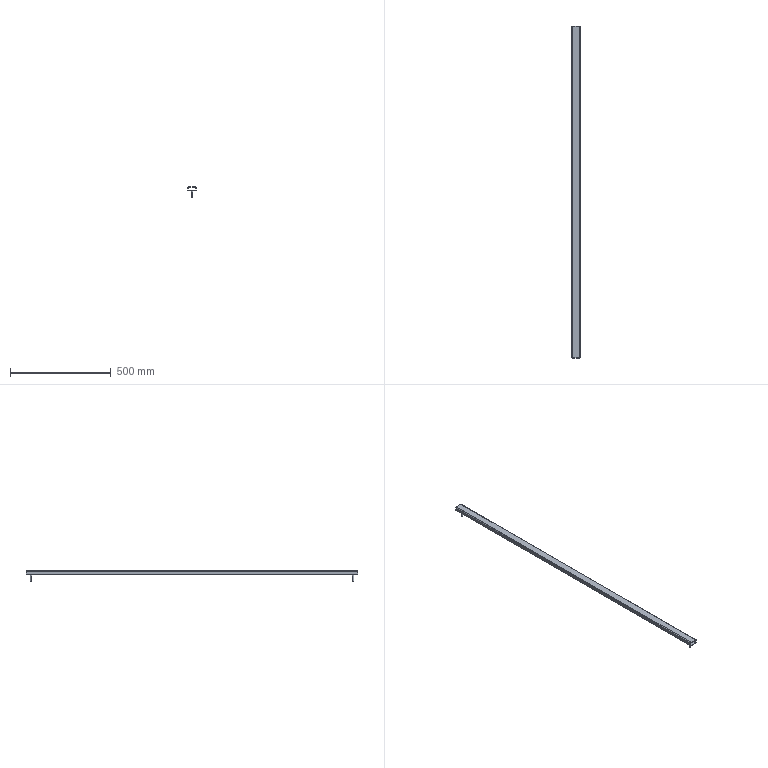Part | SolidWorks | features Extrusion 1, ICE 1 | 1 solid | 24 faces | box 40 x 1650 x 50 mm | volume 355619 mm3 | cylinder 12 | plane 12 | commonest cylinder face diameters 8 x8 4 x4
STEP:
#1=CARTESIAN_POINT('',(-4.,25.,-40.));
#2=VERTEX_POINT('',#1);
#3=CARTESIAN_POINT('',(4.,25.,-40.));
#4=VERTEX_POINT('',#3);
#5=CARTESIAN_POINT('',(0.,25.,-40.));
#6=DIRECTION('',(0.,0.,-1.));
#7=DIRECTION('',(-1.,0.,0.));
#8=AXIS2_PLACEMENT_3D('',#5,#6,#7);
#9=CIRCLE('',#8,4.);
#10=EDGE_CURVE('',#2,#4,#9,.T.);
#11=ORIENTED_EDGE('',*,*,#10,.F.);
#12=CARTESIAN_POINT('',(-4.,25.,-10.));
#13=VERTEX_POINT('',#12);
#14=CARTESIAN_POINT('',(-4.,25.,-40.));
#15=DIRECTION('',(0.,0.,1.));
#16=VECTOR('',#15,1000.);
#17=LINE('',#14,#16);
#18=EDGE_CURVE('',#2,#13,#17,.T.);
#19=ORIENTED_EDGE('',*,*,#18,.T.);
#20=CARTESIAN_POINT('',(4.,25.,-10.));
#21=VERTEX_POINT('',#20);
#22=CARTESIAN_POINT('',(0.,25.,-10.));
#23=DIRECTION('',(0.,0.,-1.));
#24=DIRECTION('',(1.,0.,0.));
#25=AXIS2_PLACEMENT_3D('',#22,#23,#24);
#26=CIRCLE('',#25,4.);
#27=EDGE_CURVE('',#13,#21,#26,.T.);
#28=ORIENTED_EDGE('',*,*,#27,.T.);
#29=CARTESIAN_POINT('',(4.,25.,-40.));
#30=DIRECTION('',(0.,0.,1.));
#31=VECTOR('',#30,1000.);
#32=LINE('',#29,#31);
#33=EDGE_CURVE('',#4,#21,#32,.T.);
#34=ORIENTED_EDGE('',*,*,#33,.F.);
#35=EDGE_LOOP('',(#11,#19,#28,#34));
#36=FACE_OUTER_BOUND('',#35,.T.);
#37=CARTESIAN_POINT('',(0.,25.,-40.));
#38=DIRECTION('',(0.,0.,1.));
#39=DIRECTION('',(1.,0.,0.));
#40=AXIS2_PLACEMENT_3D('',#37,#38,#39);
#41=CYLINDRICAL_SURFACE('',#40,4.);
#42=ADVANCED_FACE('',(#36),#41,.T.);
#43=CARTESIAN_POINT('',(-4.,1625.,-40.));
#44=VERTEX_POINT('',#43);
#45=CARTESIAN_POINT('',(4.,1625.,-40.));
#46=VERTEX_POINT('',#45);
#47=CARTESIAN_POINT('',(0.,1625.,-40.));
#48=DIRECTION('',(0.,0.,-1.));
#49=DIRECTION('',(-1.,0.,0.));
#50=AXIS2_PLACEMENT_3D('',#47,#48,#49);
#51=CIRCLE('',#50,4.);
#52=EDGE_CURVE('',#44,#46,#51,.T.);
#53=ORIENTED_EDGE('',*,*,#52,.F.);
#54=CARTESIAN_POINT('',(-4.,1625.,-10.));
#55=VERTEX_POINT('',#54);
#56=CARTESIAN_POINT('',(-4.,1625.,-40.));
#57=DIRECTION('',(0.,0.,1.));
#58=VECTOR('',#57,1000.);
#59=LINE('',#56,#58);
#60=EDGE_CURVE('',#44,#55,#59,.T.);
#61=ORIENTED_EDGE('',*,*,#60,.T.);
#62=CARTESIAN_POINT('',(4.,1625.,-10.));
#63=VERTEX_POINT('',#62);
#64=CARTESIAN_POINT('',(0.,1625.,-10.));
#65=DIRECTION('',(0.,0.,-1.));
#66=DIRECTION('',(1.,0.,0.));
#67=AXIS2_PLACEMENT_3D('',#64,#65,#66);
#68=CIRCLE('',#67,4.);
#69=EDGE_CURVE('',#55,#63,#68,.T.);
#70=ORIENTED_EDGE('',*,*,#69,.T.);
#71=CARTESIAN_POINT('',(4.,1625.,-40.));
#72=DIRECTION('',(0.,0.,1.));
#73=VECTOR('',#72,1000.);
#74=LINE('',#71,#73);
#75=EDGE_CURVE('',#46,#63,#74,.T.);
#76=ORIENTED_EDGE('',*,*,#75,.F.);
#77=EDGE_LOOP('',(#53,#61,#70,#76));
#78=FACE_OUTER_BOUND('',#77,.T.);
#79=CARTESIAN_POINT('',(0.,1625.,-40.));
#80=DIRECTION('',(0.,0.,1.));
#81=DIRECTION('',(1.,0.,0.));
#82=AXIS2_PLACEMENT_3D('',#79,#80,#81);
#83=CYLINDRICAL_SURFACE('',#82,4.);
#84=ADVANCED_FACE('',(#78),#83,.T.);
#85=CARTESIAN_POINT('',(-20.,1650.,6.));
#86=VERTEX_POINT('',#85);
#87=CARTESIAN_POINT('',(-16.,1650.,10.));
#88=VERTEX_POINT('',#87);
#89=CARTESIAN_POINT('',(-16.,1650.,6.));
#90=DIRECTION('',(0.,1.,0.));
#91=DIRECTION('',(0.,0.,-1.));
#92=AXIS2_PLACEMENT_3D('',#89,#90,#91);
#93=CIRCLE('',#92,4.);
#94=EDGE_CURVE('',#86,#88,#93,.T.);
#95=ORIENTED_EDGE('',*,*,#94,.T.);
#96=CARTESIAN_POINT('',(16.,1650.,10.));
#97=VERTEX_POINT('',#96);
#98=CARTESIAN_POINT('',(-16.,1650.,10.));
#99=DIRECTION('',(1.,0.,0.));
#100=VECTOR('',#99,1000.);
#101=LINE('',#98,#100);
#102=EDGE_CURVE('',#88,#97,#101,.T.);
#103=ORIENTED_EDGE('',*,*,#102,.T.);
#104=CARTESIAN_POINT('',(20.,1650.,6.));
#105=VERTEX_POINT('',#104);
#106=CARTESIAN_POINT('',(16.,1650.,6.));
#107=DIRECTION('',(0.,1.,0.));
#108=DIRECTION('',(0.,0.,1.));
#109=AXIS2_PLACEMENT_3D('',#106,#107,#108);
#110=CIRCLE('',#109,4.);
#111=EDGE_CURVE('',#97,#105,#110,.T.);
#112=ORIENTED_EDGE('',*,*,#111,.T.);
#113=CARTESIAN_POINT('',(20.,1650.,-6.));
#114=VERTEX_POINT('',#113);
#115=CARTESIAN_POINT('',(20.,1650.,6.));
#116=DIRECTION('',(0.,0.,-1.));
#117=VECTOR('',#116,1000.);
#118=LINE('',#115,#117);
#119=EDGE_CURVE('',#105,#114,#118,.T.);
#120=ORIENTED_EDGE('',*,*,#119,.T.);
#121=CARTESIAN_POINT('',(16.,1650.,-10.));
#122=VERTEX_POINT('',#121);
#123=CARTESIAN_POINT('',(16.,1650.,-6.));
#124=DIRECTION('',(0.,1.,0.));
#125=DIRECTION('',(0.,0.,-1.));
#126=AXIS2_PLACEMENT_3D('',#123,#124,#125);
#127=CIRCLE('',#126,4.);
#128=EDGE_CURVE('',#114,#122,#127,.T.);
#129=ORIENTED_EDGE('',*,*,#128,.T.);
#130=CARTESIAN_POINT('',(-16.,1650.,-10.));
#131=VERTEX_POINT('',#130);
#132=CARTESIAN_POINT('',(-16.,1650.,-10.));
#133=DIRECTION('',(-1.,0.,0.));
#134=VECTOR('',#133,1000.);
#135=LINE('',#132,#134);
#136=EDGE_CURVE('',#122,#131,#135,.T.);
#137=ORIENTED_EDGE('',*,*,#136,.T.);
#138=CARTESIAN_POINT('',(-20.,1650.,-6.));
#139=VERTEX_POINT('',#138);
#140=CARTESIAN_POINT('',(-16.,1650.,-6.));
#141=DIRECTION('',(0.,1.,0.));
#142=DIRECTION('',(0.,0.,-1.));
#143=AXIS2_PLACEMENT_3D('',#140,#141,#142);
#144=CIRCLE('',#143,4.);
#145=EDGE_CURVE('',#131,#139,#144,.T.);
#146=ORIENTED_EDGE('',*,*,#145,.T.);
#147=CARTESIAN_POINT('',(-20.,1650.,6.));
#148=DIRECTION('',(0.,0.,1.));
#149=VECTOR('',#148,1000.);
#150=LINE('',#147,#149);
#151=EDGE_CURVE('',#139,#86,#150,.T.);
#152=ORIENTED_EDGE('',*,*,#151,.T.);
#153=EDGE_LOOP('',(#95,#103,#112,#120,#129,#137,#146,#152));
#154=FACE_OUTER_BOUND('',#153,.T.);
#155=CARTESIAN_POINT('',(-18.,1650.,6.));
#156=VERTEX_POINT('',#155);
#157=CARTESIAN_POINT('',(-16.,1650.,8.));
#158=VERTEX_POINT('',#157);
#159=CARTESIAN_POINT('',(-16.,1650.,6.));
#160=DIRECTION('',(0.,1.,0.));
#161=DIRECTION('',(0.,0.,-1.));
#162=AXIS2_PLACEMENT_3D('',#159,#160,#161);
#163=CIRCLE('',#162,2.);
#164=EDGE_CURVE('',#156,#158,#163,.T.);
#165=ORIENTED_EDGE('',*,*,#164,.F.);
#166=CARTESIAN_POINT('',(-18.,1650.,-6.));
#167=VERTEX_POINT('',#166);
#168=CARTESIAN_POINT('',(-18.,1650.,6.));
#169=DIRECTION('',(0.,0.,1.));
#170=VECTOR('',#169,1000.);
#171=LINE('',#168,#170);
#172=EDGE_CURVE('',#167,#156,#171,.T.);
#173=ORIENTED_EDGE('',*,*,#172,.F.);
#174=CARTESIAN_POINT('',(-16.,1650.,-8.));
#175=VERTEX_POINT('',#174);
#176=CARTESIAN_POINT('',(-16.,1650.,-6.));
#177=DIRECTION('',(0.,1.,0.));
#178=DIRECTION('',(0.,0.,-1.));
#179=AXIS2_PLACEMENT_3D('',#176,#177,#178);
#180=CIRCLE('',#179,2.);
#181=EDGE_CURVE('',#175,#167,#180,.T.);
#182=ORIENTED_EDGE('',*,*,#181,.F.);
#183=CARTESIAN_POINT('',(16.,1650.,-8.));
#184=VERTEX_POINT('',#183);
#185=CARTESIAN_POINT('',(-16.,1650.,-8.));
#186=DIRECTION('',(-1.,0.,0.));
#187=VECTOR('',#186,1000.);
#188=LINE('',#185,#187);
#189=EDGE_CURVE('',#184,#175,#188,.T.);
#190=ORIENTED_EDGE('',*,*,#189,.F.);
#191=CARTESIAN_POINT('',(18.,1650.,-6.));
#192=VERTEX_POINT('',#191);
#193=CARTESIAN_POINT('',(16.,1650.,-6.));
#194=DIRECTION('',(0.,1.,0.));
#195=DIRECTION('',(0.,0.,-1.));
#196=AXIS2_PLACEMENT_3D('',#193,#194,#195);
#197=CIRCLE('',#196,2.);
#198=EDGE_CURVE('',#192,#184,#197,.T.);
#199=ORIENTED_EDGE('',*,*,#198,.F.);
#200=CARTESIAN_POINT('',(18.,1650.,6.));
#201=VERTEX_POINT('',#200);
#202=CARTESIAN_POINT('',(18.,1650.,6.));
#203=DIRECTION('',(0.,0.,-1.));
#204=VECTOR('',#203,1000.);
#205=LINE('',#202,#204);
#206=EDGE_CURVE('',#201,#192,#205,.T.);
#207=ORIENTED_EDGE('',*,*,#206,.F.);
#208=CARTESIAN_POINT('',(16.,1650.,8.));
#209=VERTEX_POINT('',#208);
#210=CARTESIAN_POINT('',(16.,1650.,6.));
#211=DIRECTION('',(0.,1.,0.));
#212=DIRECTION('',(0.,0.,1.));
#213=AXIS2_PLACEMENT_3D('',#210,#211,#212);
#214=CIRCLE('',#213,2.);
#215=EDGE_CURVE('',#209,#201,#214,.T.);
#216=ORIENTED_EDGE('',*,*,#215,.F.);
#217=CARTESIAN_POINT('',(-16.,1650.,8.));
#218=DIRECTION('',(1.,0.,0.));
#219=VECTOR('',#218,1000.);
#220=LINE('',#217,#219);
#221=EDGE_CURVE('',#158,#209,#220,.T.);
#222=ORIENTED_EDGE('',*,*,#221,.F.);
#223=EDGE_LOOP('',(#165,#173,#182,#190,#199,#207,#216,#222));
#224=FACE_BOUND('',#223,.T.);
#225=CARTESIAN_POINT('',(-16.,1650.,6.));
#226=DIRECTION('',(0.,-1.,0.));
#227=DIRECTION('',(0.,0.,-1.));
#228=AXIS2_PLACEMENT_3D('',#225,#226,#227);
#229=PLANE('',#228);
#230=ADVANCED_FACE('',(#154,#224),#229,.F.);
#231=CARTESIAN_POINT('',(-20.,0.,6.));
#232=VERTEX_POINT('',#231);
#233=CARTESIAN_POINT('',(-16.,0.,10.));
#234=VERTEX_POINT('',#233);
#235=CARTESIAN_POINT('',(-16.,0.,6.));
#236=DIRECTION('',(0.,1.,0.));
#237=DIRECTION('',(0.,0.,-1.));
#238=AXIS2_PLACEMENT_3D('',#235,#236,#237);
#239=CIRCLE('',#238,4.);
#240=EDGE_CURVE('',#232,#234,#239,.T.);
#241=ORIENTED_EDGE('',*,*,#240,.F.);
#242=CARTESIAN_POINT('',(-20.,0.,-6.));
#243=VERTEX_POINT('',#242);
#244=CARTESIAN_POINT('',(-20.,0.,6.));
#245=DIRECTION('',(0.,0.,1.));
#246=VECTOR('',#245,1000.);
#247=LINE('',#244,#246);
#248=EDGE_CURVE('',#243,#232,#247,.T.);
#249=ORIENTED_EDGE('',*,*,#248,.F.);
#250=CARTESIAN_POINT('',(-16.,0.,-10.));
#251=VERTEX_POINT('',#250);
#252=CARTESIAN_POINT('',(-16.,0.,-6.));
#253=DIRECTION('',(0.,1.,0.));
#254=DIRECTION('',(0.,0.,-1.));
#255=AXIS2_PLACEMENT_3D('',#252,#253,#254);
#256=CIRCLE('',#255,4.);
#257=EDGE_CURVE('',#251,#243,#256,.T.);
#258=ORIENTED_EDGE('',*,*,#257,.F.);
#259=CARTESIAN_POINT('',(16.,0.,-10.));
#260=VERTEX_POINT('',#259);
#261=CARTESIAN_POINT('',(-16.,0.,-10.));
#262=DIRECTION('',(-1.,0.,0.));
#263=VECTOR('',#262,1000.);
#264=LINE('',#261,#263);
#265=EDGE_CURVE('',#260,#251,#264,.T.);
#266=ORIENTED_EDGE('',*,*,#265,.F.);
#267=CARTESIAN_POINT('',(20.,0.,-6.));
#268=VERTEX_POINT('',#267);
#269=CARTESIAN_POINT('',(16.,0.,-6.));
#270=DIRECTION('',(0.,1.,0.));
#271=DIRECTION('',(0.,0.,-1.));
#272=AXIS2_PLACEMENT_3D('',#269,#270,#271);
#273=CIRCLE('',#272,4.);
#274=EDGE_CURVE('',#268,#260,#273,.T.);
#275=ORIENTED_EDGE('',*,*,#274,.F.);
#276=CARTESIAN_POINT('',(20.,0.,6.));
#277=VERTEX_POINT('',#276);
#278=CARTESIAN_POINT('',(20.,0.,6.));
#279=DIRECTION('',(0.,0.,-1.));
#280=VECTOR('',#279,1000.);
#281=LINE('',#278,#280);
#282=EDGE_CURVE('',#277,#268,#281,.T.);
#283=ORIENTED_EDGE('',*,*,#282,.F.);
#284=CARTESIAN_POINT('',(16.,0.,10.));
#285=VERTEX_POINT('',#284);
#286=CARTESIAN_POINT('',(16.,0.,6.));
#287=DIRECTION('',(0.,1.,0.));
#288=DIRECTION('',(0.,0.,1.));
#289=AXIS2_PLACEMENT_3D('',#286,#287,#288);
#290=CIRCLE('',#289,4.);
#291=EDGE_CURVE('',#285,#277,#290,.T.);
#292=ORIENTED_EDGE('',*,*,#291,.F.);
#293=CARTESIAN_POINT('',(-16.,0.,10.));
#294=DIRECTION('',(1.,0.,0.));
#295=VECTOR('',#294,1000.);
#296=LINE('',#293,#295);
#297=EDGE_CURVE('',#234,#285,#296,.T.);
#298=ORIENTED_EDGE('',*,*,#297,.F.);
#299=EDGE_LOOP('',(#241,#249,#258,#266,#275,#283,#292,#298));
#300=FACE_OUTER_BOUND('',#299,.T.);
#301=CARTESIAN_POINT('',(-18.,0.,-6.));
#302=VERTEX_POINT('',#301);
#303=CARTESIAN_POINT('',(-18.,0.,6.));
#304=VERTEX_POINT('',#303);
#305=CARTESIAN_POINT('',(-18.,0.,6.));
#306=DIRECTION('',(0.,0.,1.));
#307=VECTOR('',#306,1000.);
#308=LINE('',#305,#307);
#309=EDGE_CURVE('',#302,#304,#308,.T.);
#310=ORIENTED_EDGE('',*,*,#309,.T.);
#311=CARTESIAN_POINT('',(-16.,0.,8.));
#312=VERTEX_POINT('',#311);
#313=CARTESIAN_POINT('',(-16.,0.,6.));
#314=DIRECTION('',(0.,1.,0.));
#315=DIRECTION('',(0.,0.,-1.));
#316=AXIS2_PLACEMENT_3D('',#313,#314,#315);
#317=CIRCLE('',#316,2.);
#318=EDGE_CURVE('',#304,#312,#317,.T.);
#319=ORIENTED_EDGE('',*,*,#318,.T.);
#320=CARTESIAN_POINT('',(16.,0.,8.));
#321=VERTEX_POINT('',#320);
#322=CARTESIAN_POINT('',(-16.,0.,8.));
#323=DIRECTION('',(1.,0.,0.));
#324=VECTOR('',#323,1000.);
#325=LINE('',#322,#324);
#326=EDGE_CURVE('',#312,#321,#325,.T.);
#327=ORIENTED_EDGE('',*,*,#326,.T.);
#328=CARTESIAN_POINT('',(18.,0.,6.));
#329=VERTEX_POINT('',#328);
#330=CARTESIAN_POINT('',(16.,0.,6.));
#331=DIRECTION('',(0.,1.,0.));
#332=DIRECTION('',(0.,0.,1.));
#333=AXIS2_PLACEMENT_3D('',#330,#331,#332);
#334=CIRCLE('',#333,2.);
#335=EDGE_CURVE('',#321,#329,#334,.T.);
#336=ORIENTED_EDGE('',*,*,#335,.T.);
#337=CARTESIAN_POINT('',(18.,0.,-6.));
#338=VERTEX_POINT('',#337);
#339=CARTESIAN_POINT('',(18.,0.,6.));
#340=DIRECTION('',(0.,0.,-1.));
#341=VECTOR('',#340,1000.);
#342=LINE('',#339,#341);
#343=EDGE_CURVE('',#329,#338,#342,.T.);
#344=ORIENTED_EDGE('',*,*,#343,.T.);
#345=CARTESIAN_POINT('',(16.,0.,-8.));
#346=VERTEX_POINT('',#345);
#347=CARTESIAN_POINT('',(16.,0.,-6.));
#348=DIRECTION('',(0.,1.,0.));
#349=DIRECTION('',(0.,0.,-1.));
#350=AXIS2_PLACEMENT_3D('',#347,#348,#349);
#351=CIRCLE('',#350,2.);
#352=EDGE_CURVE('',#338,#346,#351,.T.);
#353=ORIENTED_EDGE('',*,*,#352,.T.);
#354=CARTESIAN_POINT('',(-16.,0.,-8.));
#355=VERTEX_POINT('',#354);
#356=CARTESIAN_POINT('',(-16.,0.,-8.));
#357=DIRECTION('',(-1.,0.,0.));
#358=VECTOR('',#357,1000.);
#359=LINE('',#356,#358);
#360=EDGE_CURVE('',#346,#355,#359,.T.);
#361=ORIENTED_EDGE('',*,*,#360,.T.);
#362=CARTESIAN_POINT('',(-16.,0.,-6.));
#363=DIRECTION('',(0.,1.,0.));
#364=DIRECTION('',(0.,0.,-1.));
#365=AXIS2_PLACEMENT_3D('',#362,#363,#364);
#366=CIRCLE('',#365,2.);
#367=EDGE_CURVE('',#355,#302,#366,.T.);
#368=ORIENTED_EDGE('',*,*,#367,.T.);
#369=EDGE_LOOP('',(#310,#319,#327,#336,#344,#353,#361,#368));
#370=FACE_BOUND('',#369,.T.);
#371=CARTESIAN_POINT('',(-16.,0.,6.));
#372=DIRECTION('',(0.,-1.,0.));
#373=DIRECTION('',(0.,0.,-1.));
#374=AXIS2_PLACEMENT_3D('',#371,#372,#373);
#375=PLANE('',#374);
#376=ADVANCED_FACE('',(#300,#370),#375,.T.);
#377=ORIENTED_EDGE('',*,*,#240,.T.);
#378=CARTESIAN_POINT('',(-16.,1650.,10.));
#379=DIRECTION('',(0.,-1.,0.));
#380=VECTOR('',#379,1000.);
#381=LINE('',#378,#380);
#382=EDGE_CURVE('',#88,#234,#381,.T.);
#383=ORIENTED_EDGE('',*,*,#382,.F.);
#384=ORIENTED_EDGE('',*,*,#94,.F.);
#385=CARTESIAN_POINT('',(-20.,1650.,6.));
#386=DIRECTION('',(0.,-1.,0.));
#387=VECTOR('',#386,1000.);
#388=LINE('',#385,#387);
#389=EDGE_CURVE('',#86,#232,#388,.T.);
#390=ORIENTED_EDGE('',*,*,#389,.T.);
#391=EDGE_LOOP('',(#377,#383,#384,#390));
#392=FACE_OUTER_BOUND('',#391,.T.);
#393=CARTESIAN_POINT('',(-16.,1650.,6.));
#394=DIRECTION('',(0.,-1.,0.));
#395=DIRECTION('',(0.,0.,-1.));
#396=AXIS2_PLACEMENT_3D('',#393,#394,#395);
#397=CYLINDRICAL_SURFACE('',#396,4.);
#398=ADVANCED_FACE('',(#392),#397,.T.);
#399=ORIENTED_EDGE('',*,*,#297,.T.);
#400=CARTESIAN_POINT('',(16.,1650.,10.));
#401=DIRECTION('',(0.,-1.,0.));
#402=VECTOR('',#401,1000.);
#403=LINE('',#400,#402);
#404=EDGE_CURVE('',#97,#285,#403,.T.);
#405=ORIENTED_EDGE('',*,*,#404,.F.);
#406=ORIENTED_EDGE('',*,*,#102,.F.);
#407=ORIENTED_EDGE('',*,*,#382,.T.);
#408=EDGE_LOOP('',(#399,#405,#406,#407));
#409=FACE_OUTER_BOUND('',#408,.T.);
#410=CARTESIAN_POINT('',(-16.,1650.,10.));
#411=DIRECTION('',(0.,0.,-1.));
#412=DIRECTION('',(-1.,0.,0.));
#413=AXIS2_PLACEMENT_3D('',#410,#411,#412);
#414=PLANE('',#413);
#415=ADVANCED_FACE('',(#409),#414,.F.);
#416=ORIENTED_EDGE('',*,*,#291,.T.);
#417=CARTESIAN_POINT('',(20.,1650.,6.));
#418=DIRECTION('',(0.,-1.,0.));
#419=VECTOR('',#418,1000.);
#420=LINE('',#417,#419);
#421=EDGE_CURVE('',#105,#277,#420,.T.);
#422=ORIENTED_EDGE('',*,*,#421,.F.);
#423=ORIENTED_EDGE('',*,*,#111,.F.);
#424=ORIENTED_EDGE('',*,*,#404,.T.);
#425=EDGE_LOOP('',(#416,#422,#423,#424));
#426=FACE_OUTER_BOUND('',#425,.T.);
#427=CARTESIAN_POINT('',(16.,1650.,6.));
#428=DIRECTION('',(0.,-1.,0.));
#429=DIRECTION('',(0.,0.,-1.));
#430=AXIS2_PLACEMENT_3D('',#427,#428,#429);
#431=CYLINDRICAL_SURFACE('',#430,4.);
#432=ADVANCED_FACE('',(#426),#431,.T.);
#433=ORIENTED_EDGE('',*,*,#282,.T.);
#434=CARTESIAN_POINT('',(20.,1650.,-6.));
#435=DIRECTION('',(0.,-1.,0.));
#436=VECTOR('',#435,1000.);
#437=LINE('',#434,#436);
#438=EDGE_CURVE('',#114,#268,#437,.T.);
#439=ORIENTED_EDGE('',*,*,#438,.F.);
#440=ORIENTED_EDGE('',*,*,#119,.F.);
#441=ORIENTED_EDGE('',*,*,#421,.T.);
#442=EDGE_LOOP('',(#433,#439,#440,#441));
#443=FACE_OUTER_BOUND('',#442,.T.);
#444=CARTESIAN_POINT('',(20.,1650.,6.));
#445=DIRECTION('',(-1.,0.,0.));
#446=DIRECTION('',(0.,0.,1.));
#447=AXIS2_PLACEMENT_3D('',#444,#445,#446);
#448=PLANE('',#447);
#449=ADVANCED_FACE('',(#443),#448,.F.);
#450=ORIENTED_EDGE('',*,*,#274,.T.);
#451=CARTESIAN_POINT('',(16.,1650.,-10.));
#452=DIRECTION('',(0.,-1.,0.));
#453=VECTOR('',#452,1000.);
#454=LINE('',#451,#453);
#455=EDGE_CURVE('',#122,#260,#454,.T.);
#456=ORIENTED_EDGE('',*,*,#455,.F.);
#457=ORIENTED_EDGE('',*,*,#128,.F.);
#458=ORIENTED_EDGE('',*,*,#438,.T.);
#459=EDGE_LOOP('',(#450,#456,#457,#458));
#460=FACE_OUTER_BOUND('',#459,.T.);
#461=CARTESIAN_POINT('',(16.,1650.,-6.));
#462=DIRECTION('',(0.,-1.,0.));
#463=DIRECTION('',(0.,0.,-1.));
#464=AXIS2_PLACEMENT_3D('',#461,#462,#463);
#465=CYLINDRICAL_SURFACE('',#464,4.);
#466=ADVANCED_FACE('',(#460),#465,.T.);
#467=CARTESIAN_POINT('',(0.,25.,-10.));
#468=DIRECTION('',(0.,0.,-1.));
#469=DIRECTION('',(1.,0.,0.));
#470=AXIS2_PLACEMENT_3D('',#467,#468,#469);
#471=CIRCLE('',#470,4.);
#472=EDGE_CURVE('',#21,#13,#471,.T.);
#473=ORIENTED_EDGE('',*,*,#472,.F.);
#474=ORIENTED_EDGE('',*,*,#27,.F.);
#475=EDGE_LOOP('',(#473,#474));
#476=FACE_BOUND('',#475,.T.);
#477=CARTESIAN_POINT('',(0.,1625.,-10.));
#478=DIRECTION('',(0.,0.,-1.));
#479=DIRECTION('',(1.,0.,0.));
#480=AXIS2_PLACEMENT_3D('',#477,#478,#479);
#481=CIRCLE('',#480,4.);
#482=EDGE_CURVE('',#63,#55,#481,.T.);
#483=ORIENTED_EDGE('',*,*,#482,.F.);
#484=ORIENTED_EDGE('',*,*,#69,.F.);
#485=EDGE_LOOP('',(#483,#484));
#486=FACE_BOUND('',#485,.T.);
#487=ORIENTED_EDGE('',*,*,#265,.T.);
#488=CARTESIAN_POINT('',(-16.,1650.,-10.));
#489=DIRECTION('',(0.,-1.,0.));
#490=VECTOR('',#489,1000.);
#491=LINE('',#488,#490);
#492=EDGE_CURVE('',#131,#251,#491,.T.);
#493=ORIENTED_EDGE('',*,*,#492,.F.);
#494=ORIENTED_EDGE('',*,*,#136,.F.);
#495=ORIENTED_EDGE('',*,*,#455,.T.);
#496=EDGE_LOOP('',(#487,#493,#494,#495));
#497=FACE_OUTER_BOUND('',#496,.T.);
#498=CARTESIAN_POINT('',(-16.,1650.,-10.));
#499=DIRECTION('',(0.,0.,1.));
#500=DIRECTION('',(1.,0.,0.));
#501=AXIS2_PLACEMENT_3D('',#498,#499,#500);
#502=PLANE('',#501);
#503=ADVANCED_FACE('',(#476,#486,#497),#502,.F.);
#504=ORIENTED_EDGE('',*,*,#257,.T.);
#505=CARTESIAN_POINT('',(-20.,1650.,-6.));
#506=DIRECTION('',(0.,-1.,0.));
#507=VECTOR('',#506,1000.);
#508=LINE('',#505,#507);
#509=EDGE_CURVE('',#139,#243,#508,.T.);
#510=ORIENTED_EDGE('',*,*,#509,.F.);
#511=ORIENTED_EDGE('',*,*,#145,.F.);
#512=ORIENTED_EDGE('',*,*,#492,.T.);
#513=EDGE_LOOP('',(#504,#510,#511,#512));
#514=FACE_OUTER_BOUND('',#513,.T.);
#515=CARTESIAN_POINT('',(-16.,1650.,-6.));
#516=DIRECTION('',(0.,-1.,0.));
#517=DIRECTION('',(0.,0.,-1.));
#518=AXIS2_PLACEMENT_3D('',#515,#516,#517);
#519=CYLINDRICAL_SURFACE('',#518,4.);
#520=ADVANCED_FACE('',(#514),#519,.T.);
#521=ORIENTED_EDGE('',*,*,#248,.T.);
#522=ORIENTED_EDGE('',*,*,#389,.F.);
#523=ORIENTED_EDGE('',*,*,#151,.F.);
#524=ORIENTED_EDGE('',*,*,#509,.T.);
#525=EDGE_LOOP('',(#521,#522,#523,#524));
#526=FACE_OUTER_BOUND('',#525,.T.);
#527=CARTESIAN_POINT('',(-20.,1650.,6.));
#528=DIRECTION('',(1.,0.,0.));
#529=DIRECTION('',(0.,0.,-1.));
#530=AXIS2_PLACEMENT_3D('',#527,#528,#529);
#531=PLANE('',#530);
#532=ADVANCED_FACE('',(#526),#531,.F.);
#533=ORIENTED_EDGE('',*,*,#318,.F.);
#534=CARTESIAN_POINT('',(-18.,1650.,6.));
#535=DIRECTION('',(0.,-1.,0.));
#536=VECTOR('',#535,1000.);
#537=LINE('',#534,#536);
#538=EDGE_CURVE('',#156,#304,#537,.T.);
#539=ORIENTED_EDGE('',*,*,#538,.F.);
#540=ORIENTED_EDGE('',*,*,#164,.T.);
#541=CARTESIAN_POINT('',(-16.,1650.,8.));
#542=DIRECTION('',(0.,-1.,0.));
#543=VECTOR('',#542,1000.);
#544=LINE('',#541,#543);
#545=EDGE_CURVE('',#158,#312,#544,.T.);
#546=ORIENTED_EDGE('',*,*,#545,.T.);
#547=EDGE_LOOP('',(#533,#539,#540,#546));
#548=FACE_OUTER_BOUND('',#547,.T.);
#549=CARTESIAN_POINT('',(-16.,1650.,6.));
#550=DIRECTION('',(0.,-1.,0.));
#551=DIRECTION('',(0.,0.,-1.));
#552=AXIS2_PLACEMENT_3D('',#549,#550,#551);
#553=CYLINDRICAL_SURFACE('',#552,2.);
#554=ADVANCED_FACE('',(#548),#553,.F.);
#555=ORIENTED_EDGE('',*,*,#326,.F.);
#556=ORIENTED_EDGE('',*,*,#545,.F.);
#557=ORIENTED_EDGE('',*,*,#221,.T.);
#558=CARTESIAN_POINT('',(16.,1650.,8.));
#559=DIRECTION('',(0.,-1.,0.));
#560=VECTOR('',#559,1000.);
#561=LINE('',#558,#560);
#562=EDGE_CURVE('',#209,#321,#561,.T.);
#563=ORIENTED_EDGE('',*,*,#562,.T.);
#564=EDGE_LOOP('',(#555,#556,#557,#563));
#565=FACE_OUTER_BOUND('',#564,.T.);
#566=CARTESIAN_POINT('',(-16.,1650.,8.));
#567=DIRECTION('',(0.,0.,-1.));
#568=DIRECTION('',(-1.,0.,0.));
#569=AXIS2_PLACEMENT_3D('',#566,#567,#568);
#570=PLANE('',#569);
#571=ADVANCED_FACE('',(#565),#570,.T.);
#572=ORIENTED_EDGE('',*,*,#335,.F.);
#573=ORIENTED_EDGE('',*,*,#562,.F.);
#574=ORIENTED_EDGE('',*,*,#215,.T.);
#575=CARTESIAN_POINT('',(18.,1650.,6.));
#576=DIRECTION('',(0.,-1.,0.));
#577=VECTOR('',#576,1000.);
#578=LINE('',#575,#577);
#579=EDGE_CURVE('',#201,#329,#578,.T.);
#580=ORIENTED_EDGE('',*,*,#579,.T.);
#581=EDGE_LOOP('',(#572,#573,#574,#580));
#582=FACE_OUTER_BOUND('',#581,.T.);
#583=CARTESIAN_POINT('',(16.,1650.,6.));
#584=DIRECTION('',(0.,-1.,0.));
#585=DIRECTION('',(0.,0.,-1.));
#586=AXIS2_PLACEMENT_3D('',#583,#584,#585);
#587=CYLINDRICAL_SURFACE('',#586,2.);
#588=ADVANCED_FACE('',(#582),#587,.F.);
#589=ORIENTED_EDGE('',*,*,#343,.F.);
#590=ORIENTED_EDGE('',*,*,#579,.F.);
#591=ORIENTED_EDGE('',*,*,#206,.T.);
#592=CARTESIAN_POINT('',(18.,1650.,-6.));
#593=DIRECTION('',(0.,-1.,0.));
#594=VECTOR('',#593,1000.);
#595=LINE('',#592,#594);
#596=EDGE_CURVE('',#192,#338,#595,.T.);
#597=ORIENTED_EDGE('',*,*,#596,.T.);
#598=EDGE_LOOP('',(#589,#590,#591,#597));
#599=FACE_OUTER_BOUND('',#598,.T.);
#600=CARTESIAN_POINT('',(18.,1650.,6.));
#601=DIRECTION('',(-1.,0.,0.));
#602=DIRECTION('',(0.,0.,1.));
#603=AXIS2_PLACEMENT_3D('',#600,#601,#602);
#604=PLANE('',#603);
#605=ADVANCED_FACE('',(#599),#604,.T.);
#606=ORIENTED_EDGE('',*,*,#352,.F.);
#607=ORIENTED_EDGE('',*,*,#596,.F.);
#608=ORIENTED_EDGE('',*,*,#198,.T.);
#609=CARTESIAN_POINT('',(16.,1650.,-8.));
#610=DIRECTION('',(0.,-1.,0.));
#611=VECTOR('',#610,1000.);
#612=LINE('',#609,#611);
#613=EDGE_CURVE('',#184,#346,#612,.T.);
#614=ORIENTED_EDGE('',*,*,#613,.T.);
#615=EDGE_LOOP('',(#606,#607,#608,#614));
#616=FACE_OUTER_BOUND('',#615,.T.);
#617=CARTESIAN_POINT('',(16.,1650.,-6.));
#618=DIRECTION('',(0.,-1.,0.));
#619=DIRECTION('',(0.,0.,-1.));
#620=AXIS2_PLACEMENT_3D('',#617,#618,#619);
#621=CYLINDRICAL_SURFACE('',#620,2.);
#622=ADVANCED_FACE('',(#616),#621,.F.);
#623=ORIENTED_EDGE('',*,*,#360,.F.);
#624=ORIENTED_EDGE('',*,*,#613,.F.);
#625=ORIENTED_EDGE('',*,*,#189,.T.);
#626=CARTESIAN_POINT('',(-16.,1650.,-8.));
#627=DIRECTION('',(0.,-1.,0.));
#628=VECTOR('',#627,1000.);
#629=LINE('',#626,#628);
#630=EDGE_CURVE('',#175,#355,#629,.T.);
#631=ORIENTED_EDGE('',*,*,#630,.T.);
#632=EDGE_LOOP('',(#623,#624,#625,#631));
#633=FACE_OUTER_BOUND('',#632,.T.);
#634=CARTESIAN_POINT('',(-16.,1650.,-8.));
#635=DIRECTION('',(0.,0.,1.));
#636=DIRECTION('',(1.,0.,0.));
#637=AXIS2_PLACEMENT_3D('',#634,#635,#636);
#638=PLANE('',#637);
#639=ADVANCED_FACE('',(#633),#638,.T.);
#640=ORIENTED_EDGE('',*,*,#367,.F.);
#641=ORIENTED_EDGE('',*,*,#630,.F.);
#642=ORIENTED_EDGE('',*,*,#181,.T.);
#643=CARTESIAN_POINT('',(-18.,1650.,-6.));
#644=DIRECTION('',(0.,-1.,0.));
#645=VECTOR('',#644,1000.);
#646=LINE('',#643,#645);
#647=EDGE_CURVE('',#167,#302,#646,.T.);
#648=ORIENTED_EDGE('',*,*,#647,.T.);
#649=EDGE_LOOP('',(#640,#641,#642,#648));
#650=FACE_OUTER_BOUND('',#649,.T.);
#651=CARTESIAN_POINT('',(-16.,1650.,-6.));
#652=DIRECTION('',(0.,-1.,0.));
#653=DIRECTION('',(0.,0.,-1.));
#654=AXIS2_PLACEMENT_3D('',#651,#652,#653);
#655=CYLINDRICAL_SURFACE('',#654,2.);
#656=ADVANCED_FACE('',(#650),#655,.F.);
#657=ORIENTED_EDGE('',*,*,#309,.F.);
#658=ORIENTED_EDGE('',*,*,#647,.F.);
#659=ORIENTED_EDGE('',*,*,#172,.T.);
#660=ORIENTED_EDGE('',*,*,#538,.T.);
#661=EDGE_LOOP('',(#657,#658,#659,#660));
#662=FACE_OUTER_BOUND('',#661,.T.);
#663=CARTESIAN_POINT('',(-18.,1650.,6.));
#664=DIRECTION('',(1.,0.,0.));
#665=DIRECTION('',(0.,0.,-1.));
#666=AXIS2_PLACEMENT_3D('',#663,#664,#665);
#667=PLANE('',#666);
#668=ADVANCED_FACE('',(#662),#667,.T.);
#669=ORIENTED_EDGE('',*,*,#60,.F.);
#670=CARTESIAN_POINT('',(0.,1625.,-40.));
#671=DIRECTION('',(0.,0.,-1.));
#672=DIRECTION('',(-1.,0.,0.));
#673=AXIS2_PLACEMENT_3D('',#670,#671,#672);
#674=CIRCLE('',#673,4.);
#675=EDGE_CURVE('',#46,#44,#674,.T.);
#676=ORIENTED_EDGE('',*,*,#675,.F.);
#677=ORIENTED_EDGE('',*,*,#75,.T.);
#678=ORIENTED_EDGE('',*,*,#482,.T.);
#679=EDGE_LOOP('',(#669,#676,#677,#678));
#680=FACE_OUTER_BOUND('',#679,.T.);
#681=CARTESIAN_POINT('',(0.,1625.,-40.));
#682=DIRECTION('',(0.,0.,1.));
#683=DIRECTION('',(1.,0.,0.));
#684=AXIS2_PLACEMENT_3D('',#681,#682,#683);
#685=CYLINDRICAL_SURFACE('',#684,4.);
#686=ADVANCED_FACE('',(#680),#685,.T.);
#687=ORIENTED_EDGE('',*,*,#675,.T.);
#688=ORIENTED_EDGE('',*,*,#52,.T.);
#689=EDGE_LOOP('',(#687,#688));
#690=FACE_OUTER_BOUND('',#689,.T.);
#691=CARTESIAN_POINT('',(0.,1625.,-40.));
#692=DIRECTION('',(0.,0.,-1.));
#693=DIRECTION('',(-1.,0.,0.));
#694=AXIS2_PLACEMENT_3D('',#691,#692,#693);
#695=PLANE('',#694);
#696=ADVANCED_FACE('',(#690),#695,.T.);
#697=ORIENTED_EDGE('',*,*,#18,.F.);
#698=CARTESIAN_POINT('',(0.,25.,-40.));
#699=DIRECTION('',(0.,0.,-1.));
#700=DIRECTION('',(-1.,0.,0.));
#701=AXIS2_PLACEMENT_3D('',#698,#699,#700);
#702=CIRCLE('',#701,4.);
#703=EDGE_CURVE('',#4,#2,#702,.T.);
#704=ORIENTED_EDGE('',*,*,#703,.F.);
#705=ORIENTED_EDGE('',*,*,#33,.T.);
#706=ORIENTED_EDGE('',*,*,#472,.T.);
#707=EDGE_LOOP('',(#697,#704,#705,#706));
#708=FACE_OUTER_BOUND('',#707,.T.);
#709=CARTESIAN_POINT('',(0.,25.,-40.));
#710=DIRECTION('',(0.,0.,1.));
#711=DIRECTION('',(1.,0.,0.));
#712=AXIS2_PLACEMENT_3D('',#709,#710,#711);
#713=CYLINDRICAL_SURFACE('',#712,4.);
#714=ADVANCED_FACE('',(#708),#713,.T.);
#715=ORIENTED_EDGE('',*,*,#703,.T.);
#716=ORIENTED_EDGE('',*,*,#10,.T.);
#717=EDGE_LOOP('',(#715,#716));
#718=FACE_OUTER_BOUND('',#717,.T.);
#719=CARTESIAN_POINT('',(0.,25.,-40.));
#720=DIRECTION('',(0.,0.,-1.));
#721=DIRECTION('',(-1.,0.,0.));
#722=AXIS2_PLACEMENT_3D('',#719,#720,#721);
#723=PLANE('',#722);
#724=ADVANCED_FACE('',(#718),#723,.T.);
#725=CLOSED_SHELL('',(#42,#84,#230,#376,#398,#415,#432,#449,#466,#503,#520,#532,#554,#571,#588,#605,#622,#639,#656,#668,#686,#696,#714,#724));
#726=MANIFOLD_SOLID_BREP('',#725);
#727=CARTESIAN_POINT('',(0.,0.,0.));
#728=DIRECTION('',(0.,0.,1.));
#729=DIRECTION('',(1.,0.,0.));
#730=AXIS2_PLACEMENT_3D('',#727,#728,#729);
#731=(LENGTH_UNIT()NAMED_UNIT(*)SI_UNIT(.MILLI.,.METRE.));
#732=UNCERTAINTY_MEASURE_WITH_UNIT(LENGTH_MEASURE(0.00001),#731,'','');
#733=(NAMED_UNIT(*)PLANE_ANGLE_UNIT()SI_UNIT($,.RADIAN.));
#734=(NAMED_UNIT(*)SI_UNIT($,.STERADIAN.)SOLID_ANGLE_UNIT());
#735=(GEOMETRIC_REPRESENTATION_CONTEXT(3)GLOBAL_UNCERTAINTY_ASSIGNED_CONTEXT((#732))GLOBAL_UNIT_ASSIGNED_CONTEXT((#731,#733,#734))REPRESENTATION_CONTEXT('',''));
#736=ADVANCED_BREP_SHAPE_REPRESENTATION('',(#726,#730),#735);